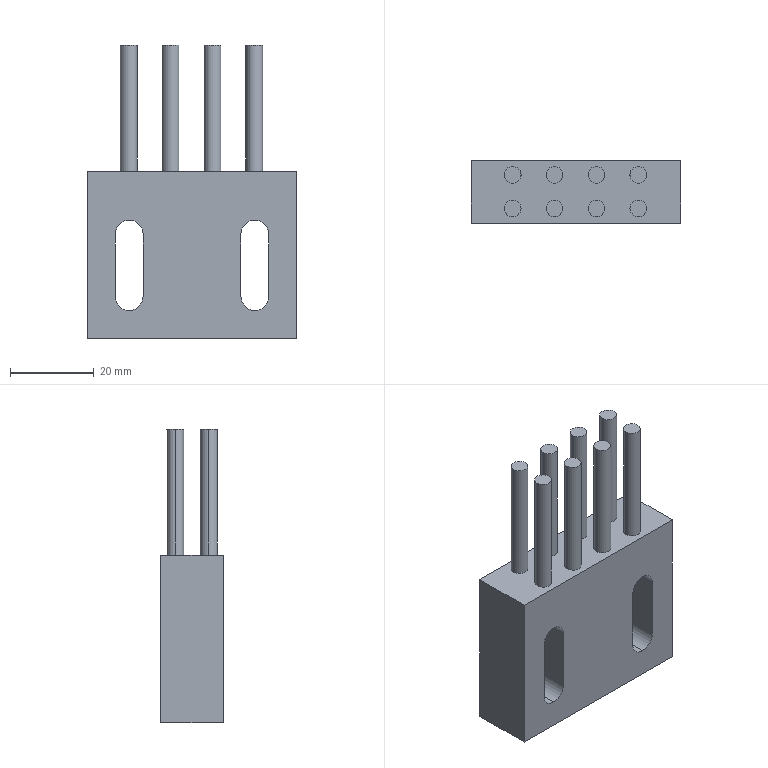Part | SolidWorks | features BaseBody 1 | 1 solid | 56 faces | box 50 x 15 x 70 mm | volume 26990 mm3 | cylinder 32 | plane 24 | commonest cylinder face diameters 4 x16 6.6 x8 11 x8